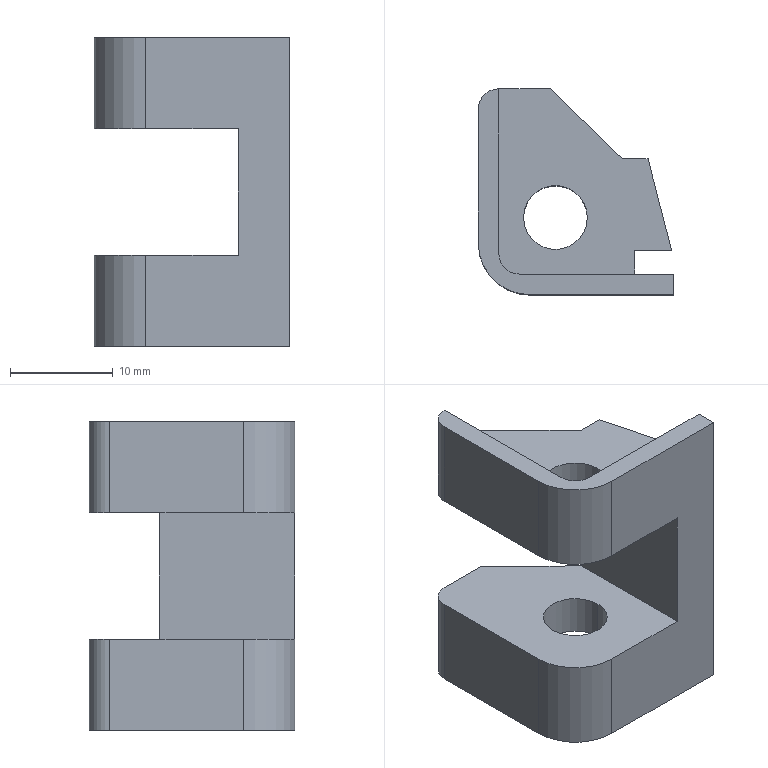Part | SolidWorks | features BaseBody 1 | 1 solid | 32 faces | box 19 x 20 x 30 mm | volume 3284 mm3 | plane 22 | cylinder 10 | commonest cylinder face diameters 4 x4 6.2 x4 10 x2
STEP:
#1=CARTESIAN_POINT('',(10.6,-12.5,-8.85));
#2=VERTEX_POINT('',#1);
#3=CARTESIAN_POINT('',(4.4,-12.5,-8.85));
#4=VERTEX_POINT('',#3);
#5=CARTESIAN_POINT('',(7.5,-12.5,-8.85));
#6=DIRECTION('',(0.,0.,-1.));
#7=DIRECTION('',(1.,0.,0.));
#8=AXIS2_PLACEMENT_3D('',#5,#6,#7);
#9=CIRCLE('',#8,3.1);
#10=EDGE_CURVE('',#2,#4,#9,.T.);
#11=ORIENTED_EDGE('',*,*,#10,.T.);
#12=CARTESIAN_POINT('',(4.4,-12.5,-5.));
#13=VERTEX_POINT('',#12);
#14=CARTESIAN_POINT('',(4.4,-12.5,-30.));
#15=DIRECTION('',(0.,0.,1.));
#16=VECTOR('',#15,1000.);
#17=LINE('',#14,#16);
#18=EDGE_CURVE('',#4,#13,#17,.T.);
#19=ORIENTED_EDGE('',*,*,#18,.T.);
#20=CARTESIAN_POINT('',(10.6,-12.5,-5.));
#21=VERTEX_POINT('',#20);
#22=CARTESIAN_POINT('',(7.5,-12.5,-5.));
#23=DIRECTION('',(0.,0.,-1.));
#24=DIRECTION('',(1.,0.,0.));
#25=AXIS2_PLACEMENT_3D('',#22,#23,#24);
#26=CIRCLE('',#25,3.1);
#27=EDGE_CURVE('',#21,#13,#26,.T.);
#28=ORIENTED_EDGE('',*,*,#27,.F.);
#29=CARTESIAN_POINT('',(10.6,-12.5,-30.));
#30=DIRECTION('',(0.,0.,1.));
#31=VECTOR('',#30,1000.);
#32=LINE('',#29,#31);
#33=EDGE_CURVE('',#2,#21,#32,.T.);
#34=ORIENTED_EDGE('',*,*,#33,.F.);
#35=EDGE_LOOP('',(#11,#19,#28,#34));
#36=FACE_OUTER_BOUND('',#35,.T.);
#37=CARTESIAN_POINT('',(7.5,-12.5,-30.));
#38=DIRECTION('',(0.,0.,1.));
#39=DIRECTION('',(1.,0.,0.));
#40=AXIS2_PLACEMENT_3D('',#37,#38,#39);
#41=CYLINDRICAL_SURFACE('',#40,3.1);
#42=ADVANCED_FACE('',(#36),#41,.F.);
#43=CARTESIAN_POINT('',(4.4,-12.5,-25.));
#44=VERTEX_POINT('',#43);
#45=CARTESIAN_POINT('',(10.6,-12.5,-25.));
#46=VERTEX_POINT('',#45);
#47=CARTESIAN_POINT('',(7.5,-12.5,-25.));
#48=DIRECTION('',(0.,0.,1.));
#49=DIRECTION('',(1.,0.,0.));
#50=AXIS2_PLACEMENT_3D('',#47,#48,#49);
#51=CIRCLE('',#50,3.1);
#52=EDGE_CURVE('',#44,#46,#51,.T.);
#53=ORIENTED_EDGE('',*,*,#52,.F.);
#54=CARTESIAN_POINT('',(4.4,-12.5,-21.15));
#55=VERTEX_POINT('',#54);
#56=CARTESIAN_POINT('',(4.4,-12.5,-30.));
#57=DIRECTION('',(0.,0.,1.));
#58=VECTOR('',#57,1000.);
#59=LINE('',#56,#58);
#60=EDGE_CURVE('',#44,#55,#59,.T.);
#61=ORIENTED_EDGE('',*,*,#60,.T.);
#62=CARTESIAN_POINT('',(10.6,-12.5,-21.15));
#63=VERTEX_POINT('',#62);
#64=CARTESIAN_POINT('',(7.5,-12.5,-21.15));
#65=DIRECTION('',(0.,0.,-1.));
#66=DIRECTION('',(1.,0.,0.));
#67=AXIS2_PLACEMENT_3D('',#64,#65,#66);
#68=CIRCLE('',#67,3.1);
#69=EDGE_CURVE('',#63,#55,#68,.T.);
#70=ORIENTED_EDGE('',*,*,#69,.F.);
#71=CARTESIAN_POINT('',(10.6,-12.5,-30.));
#72=DIRECTION('',(0.,0.,1.));
#73=VECTOR('',#72,1000.);
#74=LINE('',#71,#73);
#75=EDGE_CURVE('',#46,#63,#74,.T.);
#76=ORIENTED_EDGE('',*,*,#75,.F.);
#77=EDGE_LOOP('',(#53,#61,#70,#76));
#78=FACE_OUTER_BOUND('',#77,.T.);
#79=CARTESIAN_POINT('',(7.5,-12.5,-30.));
#80=DIRECTION('',(0.,0.,1.));
#81=DIRECTION('',(1.,0.,0.));
#82=AXIS2_PLACEMENT_3D('',#79,#80,#81);
#83=CYLINDRICAL_SURFACE('',#82,3.1);
#84=ADVANCED_FACE('',(#78),#83,.F.);
#85=CARTESIAN_POINT('',(5.,-20.,-8.85));
#86=VERTEX_POINT('',#85);
#87=CARTESIAN_POINT('',(14.,-20.,-8.85));
#88=VERTEX_POINT('',#87);
#89=CARTESIAN_POINT('',(0.,-20.,-8.85));
#90=DIRECTION('',(1.,0.,0.));
#91=VECTOR('',#90,1000.);
#92=LINE('',#89,#91);
#93=EDGE_CURVE('',#86,#88,#92,.T.);
#94=ORIENTED_EDGE('',*,*,#93,.T.);
#95=CARTESIAN_POINT('',(14.,-20.,-21.15));
#96=VERTEX_POINT('',#95);
#97=CARTESIAN_POINT('',(14.,-20.,-30.));
#98=DIRECTION('',(0.,0.,-1.));
#99=VECTOR('',#98,1000.);
#100=LINE('',#97,#99);
#101=EDGE_CURVE('',#88,#96,#100,.T.);
#102=ORIENTED_EDGE('',*,*,#101,.T.);
#103=CARTESIAN_POINT('',(5.,-20.,-21.15));
#104=VERTEX_POINT('',#103);
#105=CARTESIAN_POINT('',(0.,-20.,-21.15));
#106=DIRECTION('',(-1.,0.,0.));
#107=VECTOR('',#106,1000.);
#108=LINE('',#105,#107);
#109=EDGE_CURVE('',#96,#104,#108,.T.);
#110=ORIENTED_EDGE('',*,*,#109,.T.);
#111=CARTESIAN_POINT('',(5.,-20.,-30.));
#112=VERTEX_POINT('',#111);
#113=CARTESIAN_POINT('',(5.,-20.,-30.));
#114=DIRECTION('',(0.,0.,-1.));
#115=VECTOR('',#114,1000.);
#116=LINE('',#113,#115);
#117=EDGE_CURVE('',#104,#112,#116,.T.);
#118=ORIENTED_EDGE('',*,*,#117,.T.);
#119=CARTESIAN_POINT('',(19.,-20.,-30.));
#120=VERTEX_POINT('',#119);
#121=CARTESIAN_POINT('',(0.,-20.,-30.));
#122=DIRECTION('',(1.,0.,0.));
#123=VECTOR('',#122,1000.);
#124=LINE('',#121,#123);
#125=EDGE_CURVE('',#112,#120,#124,.T.);
#126=ORIENTED_EDGE('',*,*,#125,.T.);
#127=CARTESIAN_POINT('',(19.,-20.,0.));
#128=VERTEX_POINT('',#127);
#129=CARTESIAN_POINT('',(19.,-20.,-30.));
#130=DIRECTION('',(0.,0.,1.));
#131=VECTOR('',#130,1000.);
#132=LINE('',#129,#131);
#133=EDGE_CURVE('',#120,#128,#132,.T.);
#134=ORIENTED_EDGE('',*,*,#133,.T.);
#135=CARTESIAN_POINT('',(5.,-20.,0.));
#136=VERTEX_POINT('',#135);
#137=CARTESIAN_POINT('',(0.,-20.,0.));
#138=DIRECTION('',(-1.,0.,0.));
#139=VECTOR('',#138,1000.);
#140=LINE('',#137,#139);
#141=EDGE_CURVE('',#128,#136,#140,.T.);
#142=ORIENTED_EDGE('',*,*,#141,.T.);
#143=CARTESIAN_POINT('',(5.,-20.,-30.));
#144=DIRECTION('',(0.,0.,-1.));
#145=VECTOR('',#144,1000.);
#146=LINE('',#143,#145);
#147=EDGE_CURVE('',#136,#86,#146,.T.);
#148=ORIENTED_EDGE('',*,*,#147,.T.);
#149=EDGE_LOOP('',(#94,#102,#110,#118,#126,#134,#142,#148));
#150=FACE_OUTER_BOUND('',#149,.T.);
#151=CARTESIAN_POINT('',(0.,-20.,-30.));
#152=DIRECTION('',(0.,-1.,0.));
#153=DIRECTION('',(0.,0.,-1.));
#154=AXIS2_PLACEMENT_3D('',#151,#152,#153);
#155=PLANE('',#154);
#156=ADVANCED_FACE('',(#150),#155,.T.);
#157=CARTESIAN_POINT('',(14.,-6.8,-8.85));
#158=VERTEX_POINT('',#157);
#159=CARTESIAN_POINT('',(14.,0.,-8.85));
#160=DIRECTION('',(0.,1.,0.));
#161=VECTOR('',#160,1000.);
#162=LINE('',#159,#161);
#163=EDGE_CURVE('',#88,#158,#162,.T.);
#164=ORIENTED_EDGE('',*,*,#163,.T.);
#165=CARTESIAN_POINT('',(14.,-6.8,-21.15));
#166=VERTEX_POINT('',#165);
#167=CARTESIAN_POINT('',(14.,-6.8,-8.85));
#168=DIRECTION('',(0.,0.,-1.));
#169=VECTOR('',#168,1000.);
#170=LINE('',#167,#169);
#171=EDGE_CURVE('',#158,#166,#170,.T.);
#172=ORIENTED_EDGE('',*,*,#171,.T.);
#173=CARTESIAN_POINT('',(14.,0.,-21.15));
#174=DIRECTION('',(0.,-1.,0.));
#175=VECTOR('',#174,1000.);
#176=LINE('',#173,#175);
#177=EDGE_CURVE('',#166,#96,#176,.T.);
#178=ORIENTED_EDGE('',*,*,#177,.T.);
#179=ORIENTED_EDGE('',*,*,#101,.F.);
#180=EDGE_LOOP('',(#164,#172,#178,#179));
#181=FACE_OUTER_BOUND('',#180,.T.);
#182=CARTESIAN_POINT('',(14.,0.,-8.85));
#183=DIRECTION('',(-1.,0.,0.));
#184=DIRECTION('',(0.,-1.,0.));
#185=AXIS2_PLACEMENT_3D('',#182,#183,#184);
#186=PLANE('',#185);
#187=ADVANCED_FACE('',(#181),#186,.T.);
#188=CARTESIAN_POINT('',(2.,0.,-8.85));
#189=VERTEX_POINT('',#188);
#190=CARTESIAN_POINT('',(0.,-2.,-8.85));
#191=VERTEX_POINT('',#190);
#192=CARTESIAN_POINT('',(2.,-2.,-8.85));
#193=DIRECTION('',(0.,0.,1.));
#194=DIRECTION('',(1.,0.,0.));
#195=AXIS2_PLACEMENT_3D('',#192,#193,#194);
#196=CIRCLE('',#195,2.);
#197=EDGE_CURVE('',#189,#191,#196,.T.);
#198=ORIENTED_EDGE('',*,*,#197,.F.);
#199=CARTESIAN_POINT('',(7.,0.,-8.85));
#200=VERTEX_POINT('',#199);
#201=CARTESIAN_POINT('',(0.,0.,-8.85));
#202=DIRECTION('',(-1.,0.,0.));
#203=VECTOR('',#202,1000.);
#204=LINE('',#201,#203);
#205=EDGE_CURVE('',#200,#189,#204,.T.);
#206=ORIENTED_EDGE('',*,*,#205,.F.);
#207=CARTESIAN_POINT('',(14.,-6.8,-8.85));
#208=DIRECTION('',(-0.7173,0.6968,0.));
#209=VECTOR('',#208,1000.);
#210=LINE('',#207,#209);
#211=EDGE_CURVE('',#158,#200,#210,.T.);
#212=ORIENTED_EDGE('',*,*,#211,.F.);
#213=ORIENTED_EDGE('',*,*,#163,.F.);
#214=ORIENTED_EDGE('',*,*,#93,.F.);
#215=CARTESIAN_POINT('',(0.,-15.,-8.85));
#216=VERTEX_POINT('',#215);
#217=CARTESIAN_POINT('',(5.,-15.,-8.85));
#218=DIRECTION('',(0.,0.,1.));
#219=DIRECTION('',(1.,0.,0.));
#220=AXIS2_PLACEMENT_3D('',#217,#218,#219);
#221=CIRCLE('',#220,5.);
#222=EDGE_CURVE('',#216,#86,#221,.T.);
#223=ORIENTED_EDGE('',*,*,#222,.F.);
#224=CARTESIAN_POINT('',(0.,0.,-8.85));
#225=DIRECTION('',(0.,-1.,0.));
#226=VECTOR('',#225,1000.);
#227=LINE('',#224,#226);
#228=EDGE_CURVE('',#191,#216,#227,.T.);
#229=ORIENTED_EDGE('',*,*,#228,.F.);
#230=EDGE_LOOP('',(#198,#206,#212,#213,#214,#223,#229));
#231=FACE_OUTER_BOUND('',#230,.T.);
#232=ORIENTED_EDGE('',*,*,#10,.F.);
#233=CARTESIAN_POINT('',(7.5,-12.5,-8.85));
#234=DIRECTION('',(0.,0.,-1.));
#235=DIRECTION('',(1.,0.,0.));
#236=AXIS2_PLACEMENT_3D('',#233,#234,#235);
#237=CIRCLE('',#236,3.1);
#238=EDGE_CURVE('',#4,#2,#237,.T.);
#239=ORIENTED_EDGE('',*,*,#238,.F.);
#240=EDGE_LOOP('',(#232,#239));
#241=FACE_BOUND('',#240,.T.);
#242=CARTESIAN_POINT('',(0.,0.,-8.85));
#243=DIRECTION('',(0.,0.,1.));
#244=DIRECTION('',(1.,0.,0.));
#245=AXIS2_PLACEMENT_3D('',#242,#243,#244);
#246=PLANE('',#245);
#247=ADVANCED_FACE('',(#231,#241),#246,.F.);
#248=CARTESIAN_POINT('',(0.,-15.,0.));
#249=VERTEX_POINT('',#248);
#250=CARTESIAN_POINT('',(5.,-15.,0.));
#251=DIRECTION('',(0.,0.,-1.));
#252=DIRECTION('',(1.,0.,0.));
#253=AXIS2_PLACEMENT_3D('',#250,#251,#252);
#254=CIRCLE('',#253,5.);
#255=EDGE_CURVE('',#136,#249,#254,.T.);
#256=ORIENTED_EDGE('',*,*,#255,.T.);
#257=CARTESIAN_POINT('',(0.,-15.,-30.));
#258=DIRECTION('',(0.,0.,-1.));
#259=VECTOR('',#258,1000.);
#260=LINE('',#257,#259);
#261=EDGE_CURVE('',#249,#216,#260,.T.);
#262=ORIENTED_EDGE('',*,*,#261,.T.);
#263=ORIENTED_EDGE('',*,*,#222,.T.);
#264=ORIENTED_EDGE('',*,*,#147,.F.);
#265=EDGE_LOOP('',(#256,#262,#263,#264));
#266=FACE_OUTER_BOUND('',#265,.T.);
#267=CARTESIAN_POINT('',(5.,-15.,-30.));
#268=DIRECTION('',(0.,0.,1.));
#269=DIRECTION('',(1.,0.,0.));
#270=AXIS2_PLACEMENT_3D('',#267,#268,#269);
#271=CYLINDRICAL_SURFACE('',#270,5.);
#272=ADVANCED_FACE('',(#266),#271,.T.);
#273=CARTESIAN_POINT('',(0.,-2.,0.));
#274=VERTEX_POINT('',#273);
#275=CARTESIAN_POINT('',(2.,0.,0.));
#276=VERTEX_POINT('',#275);
#277=CARTESIAN_POINT('',(2.,-2.,0.));
#278=DIRECTION('',(0.,0.,-1.));
#279=DIRECTION('',(1.,0.,0.));
#280=AXIS2_PLACEMENT_3D('',#277,#278,#279);
#281=CIRCLE('',#280,2.);
#282=EDGE_CURVE('',#274,#276,#281,.T.);
#283=ORIENTED_EDGE('',*,*,#282,.F.);
#284=CARTESIAN_POINT('',(0.,0.,0.));
#285=DIRECTION('',(0.,1.,0.));
#286=VECTOR('',#285,1000.);
#287=LINE('',#284,#286);
#288=EDGE_CURVE('',#249,#274,#287,.T.);
#289=ORIENTED_EDGE('',*,*,#288,.F.);
#290=ORIENTED_EDGE('',*,*,#255,.F.);
#291=ORIENTED_EDGE('',*,*,#141,.F.);
#292=CARTESIAN_POINT('',(19.,-18.,0.));
#293=VERTEX_POINT('',#292);
#294=CARTESIAN_POINT('',(19.,0.,0.));
#295=DIRECTION('',(0.,-1.,0.));
#296=VECTOR('',#295,1000.);
#297=LINE('',#294,#296);
#298=EDGE_CURVE('',#293,#128,#297,.T.);
#299=ORIENTED_EDGE('',*,*,#298,.F.);
#300=CARTESIAN_POINT('',(4.,-18.,0.));
#301=VERTEX_POINT('',#300);
#302=CARTESIAN_POINT('',(0.,-18.,0.));
#303=DIRECTION('',(1.,0.,0.));
#304=VECTOR('',#303,1000.);
#305=LINE('',#302,#304);
#306=EDGE_CURVE('',#301,#293,#305,.T.);
#307=ORIENTED_EDGE('',*,*,#306,.F.);
#308=CARTESIAN_POINT('',(2.,-16.,0.));
#309=VERTEX_POINT('',#308);
#310=CARTESIAN_POINT('',(4.,-16.,0.));
#311=DIRECTION('',(0.,0.,1.));
#312=DIRECTION('',(-1.,0.,0.));
#313=AXIS2_PLACEMENT_3D('',#310,#311,#312);
#314=CIRCLE('',#313,2.);
#315=EDGE_CURVE('',#309,#301,#314,.T.);
#316=ORIENTED_EDGE('',*,*,#315,.F.);
#317=CARTESIAN_POINT('',(2.,0.,0.));
#318=DIRECTION('',(0.,-1.,0.));
#319=VECTOR('',#318,1000.);
#320=LINE('',#317,#319);
#321=EDGE_CURVE('',#276,#309,#320,.T.);
#322=ORIENTED_EDGE('',*,*,#321,.F.);
#323=EDGE_LOOP('',(#283,#289,#290,#291,#299,#307,#316,#322));
#324=FACE_OUTER_BOUND('',#323,.T.);
#325=CARTESIAN_POINT('',(0.,0.,0.));
#326=DIRECTION('',(0.,0.,-1.));
#327=DIRECTION('',(-1.,0.,0.));
#328=AXIS2_PLACEMENT_3D('',#325,#326,#327);
#329=PLANE('',#328);
#330=ADVANCED_FACE('',(#324),#329,.F.);
#331=CARTESIAN_POINT('',(19.,-18.,-30.));
#332=VERTEX_POINT('',#331);
#333=CARTESIAN_POINT('',(19.,-18.,-30.));
#334=DIRECTION('',(0.,1.,0.));
#335=VECTOR('',#334,1000.);
#336=LINE('',#333,#335);
#337=EDGE_CURVE('',#120,#332,#336,.T.);
#338=ORIENTED_EDGE('',*,*,#337,.T.);
#339=CARTESIAN_POINT('',(19.,-18.,-30.));
#340=DIRECTION('',(0.,0.,1.));
#341=VECTOR('',#340,1000.);
#342=LINE('',#339,#341);
#343=EDGE_CURVE('',#332,#293,#342,.T.);
#344=ORIENTED_EDGE('',*,*,#343,.T.);
#345=ORIENTED_EDGE('',*,*,#298,.T.);
#346=ORIENTED_EDGE('',*,*,#133,.F.);
#347=EDGE_LOOP('',(#338,#344,#345,#346));
#348=FACE_OUTER_BOUND('',#347,.T.);
#349=CARTESIAN_POINT('',(19.,-18.,-30.));
#350=DIRECTION('',(1.,0.,0.));
#351=DIRECTION('',(0.,0.,-1.));
#352=AXIS2_PLACEMENT_3D('',#349,#350,#351);
#353=PLANE('',#352);
#354=ADVANCED_FACE('',(#348),#353,.T.);
#355=ORIENTED_EDGE('',*,*,#125,.F.);
#356=CARTESIAN_POINT('',(0.,-15.,-30.));
#357=VERTEX_POINT('',#356);
#358=CARTESIAN_POINT('',(5.,-15.,-30.));
#359=DIRECTION('',(0.,0.,-1.));
#360=DIRECTION('',(1.,0.,0.));
#361=AXIS2_PLACEMENT_3D('',#358,#359,#360);
#362=CIRCLE('',#361,5.);
#363=EDGE_CURVE('',#112,#357,#362,.T.);
#364=ORIENTED_EDGE('',*,*,#363,.T.);
#365=CARTESIAN_POINT('',(0.,-2.,-30.));
#366=VERTEX_POINT('',#365);
#367=CARTESIAN_POINT('',(0.,0.,-30.));
#368=DIRECTION('',(0.,1.,0.));
#369=VECTOR('',#368,1000.);
#370=LINE('',#367,#369);
#371=EDGE_CURVE('',#357,#366,#370,.T.);
#372=ORIENTED_EDGE('',*,*,#371,.T.);
#373=CARTESIAN_POINT('',(2.,0.,-30.));
#374=VERTEX_POINT('',#373);
#375=CARTESIAN_POINT('',(2.,-2.,-30.));
#376=DIRECTION('',(0.,0.,-1.));
#377=DIRECTION('',(1.,0.,0.));
#378=AXIS2_PLACEMENT_3D('',#375,#376,#377);
#379=CIRCLE('',#378,2.);
#380=EDGE_CURVE('',#366,#374,#379,.T.);
#381=ORIENTED_EDGE('',*,*,#380,.T.);
#382=CARTESIAN_POINT('',(2.,-16.,-30.));
#383=VERTEX_POINT('',#382);
#384=CARTESIAN_POINT('',(2.,0.,-30.));
#385=DIRECTION('',(0.,-1.,0.));
#386=VECTOR('',#385,1000.);
#387=LINE('',#384,#386);
#388=EDGE_CURVE('',#374,#383,#387,.T.);
#389=ORIENTED_EDGE('',*,*,#388,.T.);
#390=CARTESIAN_POINT('',(4.,-18.,-30.));
#391=VERTEX_POINT('',#390);
#392=CARTESIAN_POINT('',(4.,-16.,-30.));
#393=DIRECTION('',(0.,0.,1.));
#394=DIRECTION('',(-1.,0.,0.));
#395=AXIS2_PLACEMENT_3D('',#392,#393,#394);
#396=CIRCLE('',#395,2.);
#397=EDGE_CURVE('',#383,#391,#396,.T.);
#398=ORIENTED_EDGE('',*,*,#397,.T.);
#399=CARTESIAN_POINT('',(0.,-18.,-30.));
#400=DIRECTION('',(1.,0.,0.));
#401=VECTOR('',#400,1000.);
#402=LINE('',#399,#401);
#403=EDGE_CURVE('',#391,#332,#402,.T.);
#404=ORIENTED_EDGE('',*,*,#403,.T.);
#405=ORIENTED_EDGE('',*,*,#337,.F.);
#406=EDGE_LOOP('',(#355,#364,#372,#381,#389,#398,#404,#405));
#407=FACE_OUTER_BOUND('',#406,.T.);
#408=CARTESIAN_POINT('',(0.,0.,-30.));
#409=DIRECTION('',(0.,0.,-1.));
#410=DIRECTION('',(-1.,0.,0.));
#411=AXIS2_PLACEMENT_3D('',#408,#409,#410);
#412=PLANE('',#411);
#413=ADVANCED_FACE('',(#407),#412,.T.);
#414=CARTESIAN_POINT('',(0.,-15.,-21.15));
#415=VERTEX_POINT('',#414);
#416=CARTESIAN_POINT('',(5.,-15.,-21.15));
#417=DIRECTION('',(0.,0.,-1.));
#418=DIRECTION('',(1.,0.,0.));
#419=AXIS2_PLACEMENT_3D('',#416,#417,#418);
#420=CIRCLE('',#419,5.);
#421=EDGE_CURVE('',#104,#415,#420,.T.);
#422=ORIENTED_EDGE('',*,*,#421,.T.);
#423=CARTESIAN_POINT('',(0.,-15.,-30.));
#424=DIRECTION('',(0.,0.,-1.));
#425=VECTOR('',#424,1000.);
#426=LINE('',#423,#425);
#427=EDGE_CURVE('',#415,#357,#426,.T.);
#428=ORIENTED_EDGE('',*,*,#427,.T.);
#429=ORIENTED_EDGE('',*,*,#363,.F.);
#430=ORIENTED_EDGE('',*,*,#117,.F.);
#431=EDGE_LOOP('',(#422,#428,#429,#430));
#432=FACE_OUTER_BOUND('',#431,.T.);
#433=CARTESIAN_POINT('',(5.,-15.,-30.));
#434=DIRECTION('',(0.,0.,1.));
#435=DIRECTION('',(1.,0.,0.));
#436=AXIS2_PLACEMENT_3D('',#433,#434,#435);
#437=CYLINDRICAL_SURFACE('',#436,5.);
#438=ADVANCED_FACE('',(#432),#437,.T.);
#439=ORIENTED_EDGE('',*,*,#177,.F.);
#440=CARTESIAN_POINT('',(7.,0.,-21.15));
#441=VERTEX_POINT('',#440);
#442=CARTESIAN_POINT('',(14.,-6.8,-21.15));
#443=DIRECTION('',(-0.7173,0.6968,0.));
#444=VECTOR('',#443,1000.);
#445=LINE('',#442,#444);
#446=EDGE_CURVE('',#166,#441,#445,.T.);
#447=ORIENTED_EDGE('',*,*,#446,.T.);
#448=CARTESIAN_POINT('',(2.,0.,-21.15));
#449=VERTEX_POINT('',#448);
#450=CARTESIAN_POINT('',(0.,0.,-21.15));
#451=DIRECTION('',(-1.,0.,0.));
#452=VECTOR('',#451,1000.);
#453=LINE('',#450,#452);
#454=EDGE_CURVE('',#441,#449,#453,.T.);
#455=ORIENTED_EDGE('',*,*,#454,.T.);
#456=CARTESIAN_POINT('',(0.,-2.,-21.15));
#457=VERTEX_POINT('',#456);
#458=CARTESIAN_POINT('',(2.,-2.,-21.15));
#459=DIRECTION('',(0.,0.,1.));
#460=DIRECTION('',(1.,0.,0.));
#461=AXIS2_PLACEMENT_3D('',#458,#459,#460);
#462=CIRCLE('',#461,2.);
#463=EDGE_CURVE('',#449,#457,#462,.T.);
#464=ORIENTED_EDGE('',*,*,#463,.T.);
#465=CARTESIAN_POINT('',(0.,0.,-21.15));
#466=DIRECTION('',(0.,-1.,0.));
#467=VECTOR('',#466,1000.);
#468=LINE('',#465,#467);
#469=EDGE_CURVE('',#457,#415,#468,.T.);
#470=ORIENTED_EDGE('',*,*,#469,.T.);
#471=ORIENTED_EDGE('',*,*,#421,.F.);
#472=ORIENTED_EDGE('',*,*,#109,.F.);
#473=EDGE_LOOP('',(#439,#447,#455,#464,#470,#471,#472));
#474=FACE_OUTER_BOUND('',#473,.T.);
#475=ORIENTED_EDGE('',*,*,#69,.T.);
#476=CARTESIAN_POINT('',(7.5,-12.5,-21.15));
#477=DIRECTION('',(0.,0.,-1.));
#478=DIRECTION('',(1.,0.,0.));
#479=AXIS2_PLACEMENT_3D('',#476,#477,#478);
#480=CIRCLE('',#479,3.1);
#481=EDGE_CURVE('',#55,#63,#480,.T.);
#482=ORIENTED_EDGE('',*,*,#481,.T.);
#483=EDGE_LOOP('',(#475,#482));
#484=FACE_BOUND('',#483,.T.);
#485=CARTESIAN_POINT('',(0.,0.,-21.15));
#486=DIRECTION('',(0.,0.,1.));
#487=DIRECTION('',(1.,0.,0.));
#488=AXIS2_PLACEMENT_3D('',#485,#486,#487);
#489=PLANE('',#488);
#490=ADVANCED_FACE('',(#474,#484),#489,.T.);
#491=CARTESIAN_POINT('',(16.5,-6.8,-5.));
#492=VERTEX_POINT('',#491);
#493=CARTESIAN_POINT('',(16.5,-6.8,-25.));
#494=VERTEX_POINT('',#493);
#495=CARTESIAN_POINT('',(16.5,-6.8,-25.));
#496=DIRECTION('',(0.,0.,-1.));
#497=VECTOR('',#496,1000.);
#498=LINE('',#495,#497);
#499=EDGE_CURVE('',#492,#494,#498,.T.);
#500=ORIENTED_EDGE('',*,*,#499,.T.);
#501=CARTESIAN_POINT('',(14.,-6.8,-25.));
#502=VERTEX_POINT('',#501);
#503=CARTESIAN_POINT('',(14.,-6.8,-25.));
#504=DIRECTION('',(-1.,0.,0.));
#505=VECTOR('',#504,1000.);
#506=LINE('',#503,#505);
#507=EDGE_CURVE('',#494,#502,#506,.T.);
#508=ORIENTED_EDGE('',*,*,#507,.T.);
#509=CARTESIAN_POINT('',(14.,-6.8,-25.));
#510=DIRECTION('',(0.,0.,1.));
#511=VECTOR('',#510,1000.);
#512=LINE('',#509,#511);
#513=EDGE_CURVE('',#502,#166,#512,.T.);
#514=ORIENTED_EDGE('',*,*,#513,.T.);
#515=ORIENTED_EDGE('',*,*,#171,.F.);
#516=CARTESIAN_POINT('',(14.,-6.8,-5.));
#517=VERTEX_POINT('',#516);
#518=CARTESIAN_POINT('',(14.,-6.8,-25.));
#519=DIRECTION('',(0.,0.,1.));
#520=VECTOR('',#519,1000.);
#521=LINE('',#518,#520);
#522=EDGE_CURVE('',#158,#517,#521,.T.);
#523=ORIENTED_EDGE('',*,*,#522,.T.);
#524=CARTESIAN_POINT('',(14.,-6.8,-5.));
#525=DIRECTION('',(1.,0.,0.));
#526=VECTOR('',#525,1000.);
#527=LINE('',#524,#526);
#528=EDGE_CURVE('',#517,#492,#527,.T.);
#529=ORIENTED_EDGE('',*,*,#528,.T.);
#530=EDGE_LOOP('',(#500,#508,#514,#515,#523,#529));
#531=FACE_OUTER_BOUND('',#530,.T.);
#532=CARTESIAN_POINT('',(14.,-6.8,-25.));
#533=DIRECTION('',(0.,1.,0.));
#534=DIRECTION('',(0.,0.,1.));
#535=AXIS2_PLACEMENT_3D('',#532,#533,#534);
#536=PLANE('',#535);
#537=ADVANCED_FACE('',(#531),#536,.T.);
#538=ORIENTED_EDGE('',*,*,#228,.T.);
#539=ORIENTED_EDGE('',*,*,#261,.F.);
#540=ORIENTED_EDGE('',*,*,#288,.T.);
#541=CARTESIAN_POINT('',(0.,-2.,-30.));
#542=DIRECTION('',(0.,0.,-1.));
#543=VECTOR('',#542,1000.);
#544=LINE('',#541,#543);
#545=EDGE_CURVE('',#274,#191,#544,.T.);
#546=ORIENTED_EDGE('',*,*,#545,.T.);
#547=EDGE_LOOP('',(#538,#539,#540,#546));
#548=FACE_OUTER_BOUND('',#547,.T.);
#549=CARTESIAN_POINT('',(0.,0.,-30.));
#550=DIRECTION('',(-1.,0.,0.));
#551=DIRECTION('',(0.,-1.,0.));
#552=AXIS2_PLACEMENT_3D('',#549,#550,#551);
#553=PLANE('',#552);
#554=ADVANCED_FACE('',(#548),#553,.T.);
#555=CARTESIAN_POINT('',(2.,0.,-5.));
#556=VERTEX_POINT('',#555);
#557=CARTESIAN_POINT('',(2.,0.,-30.));
#558=DIRECTION('',(0.,0.,-1.));
#559=VECTOR('',#558,1000.);
#560=LINE('',#557,#559);
#561=EDGE_CURVE('',#276,#556,#560,.T.);
#562=ORIENTED_EDGE('',*,*,#561,.T.);
#563=CARTESIAN_POINT('',(2.,0.,-30.));
#564=DIRECTION('',(0.,0.,-1.));
#565=VECTOR('',#564,1000.);
#566=LINE('',#563,#565);
#567=EDGE_CURVE('',#556,#189,#566,.T.);
#568=ORIENTED_EDGE('',*,*,#567,.T.);
#569=ORIENTED_EDGE('',*,*,#197,.T.);
#570=ORIENTED_EDGE('',*,*,#545,.F.);
#571=ORIENTED_EDGE('',*,*,#282,.T.);
#572=EDGE_LOOP('',(#562,#568,#569,#570,#571));
#573=FACE_OUTER_BOUND('',#572,.T.);
#574=CARTESIAN_POINT('',(2.,-2.,-30.));
#575=DIRECTION('',(0.,0.,1.));
#576=DIRECTION('',(1.,0.,0.));
#577=AXIS2_PLACEMENT_3D('',#574,#575,#576);
#578=CYLINDRICAL_SURFACE('',#577,2.);
#579=ADVANCED_FACE('',(#573),#578,.T.);
#580=CARTESIAN_POINT('',(7.,0.,-5.));
#581=VERTEX_POINT('',#580);
#582=CARTESIAN_POINT('',(0.,0.,-5.));
#583=DIRECTION('',(1.,0.,0.));
#584=VECTOR('',#583,1000.);
#585=LINE('',#582,#584);
#586=EDGE_CURVE('',#556,#581,#585,.T.);
#587=ORIENTED_EDGE('',*,*,#586,.T.);
#588=CARTESIAN_POINT('',(7.,0.,-30.));
#589=DIRECTION('',(0.,0.,-1.));
#590=VECTOR('',#589,1000.);
#591=LINE('',#588,#590);
#592=EDGE_CURVE('',#581,#200,#591,.T.);
#593=ORIENTED_EDGE('',*,*,#592,.T.);
#594=ORIENTED_EDGE('',*,*,#205,.T.);
#595=ORIENTED_EDGE('',*,*,#567,.F.);
#596=EDGE_LOOP('',(#587,#593,#594,#595));
#597=FACE_OUTER_BOUND('',#596,.T.);
#598=CARTESIAN_POINT('',(0.,0.,-30.));
#599=DIRECTION('',(0.,1.,0.));
#600=DIRECTION('',(0.,0.,1.));
#601=AXIS2_PLACEMENT_3D('',#598,#599,#600);
#602=PLANE('',#601);
#603=ADVANCED_FACE('',(#597),#602,.T.);
#604=CARTESIAN_POINT('',(7.,0.,-5.));
#605=DIRECTION('',(0.7173,-0.6968,0.));
#606=VECTOR('',#605,1000.);
#607=LINE('',#604,#606);
#608=EDGE_CURVE('',#581,#517,#607,.T.);
#609=ORIENTED_EDGE('',*,*,#608,.T.);
#610=ORIENTED_EDGE('',*,*,#522,.F.);
#611=ORIENTED_EDGE('',*,*,#211,.T.);
#612=ORIENTED_EDGE('',*,*,#592,.F.);
#613=EDGE_LOOP('',(#609,#610,#611,#612));
#614=FACE_OUTER_BOUND('',#613,.T.);
#615=CARTESIAN_POINT('',(7.,0.,-25.));
#616=DIRECTION('',(0.6968,0.7173,0.));
#617=DIRECTION('',(-0.7173,0.6968,0.));
#618=AXIS2_PLACEMENT_3D('',#615,#616,#617);
#619=PLANE('',#618);
#620=ADVANCED_FACE('',(#614),#619,.T.);
#621=ORIENTED_EDGE('',*,*,#18,.F.);
#622=ORIENTED_EDGE('',*,*,#238,.T.);
#623=ORIENTED_EDGE('',*,*,#33,.T.);
#624=CARTESIAN_POINT('',(7.5,-12.5,-5.));
#625=DIRECTION('',(0.,0.,-1.));
#626=DIRECTION('',(1.,0.,0.));
#627=AXIS2_PLACEMENT_3D('',#624,#625,#626);
#628=CIRCLE('',#627,3.1);
#629=EDGE_CURVE('',#13,#21,#628,.T.);
#630=ORIENTED_EDGE('',*,*,#629,.F.);
#631=EDGE_LOOP('',(#621,#622,#623,#630));
#632=FACE_OUTER_BOUND('',#631,.T.);
#633=CARTESIAN_POINT('',(7.5,-12.5,-30.));
#634=DIRECTION('',(0.,0.,1.));
#635=DIRECTION('',(1.,0.,0.));
#636=AXIS2_PLACEMENT_3D('',#633,#634,#635);
#637=CYLINDRICAL_SURFACE('',#636,3.1);
#638=ADVANCED_FACE('',(#632),#637,.F.);
#639=CARTESIAN_POINT('',(2.,-16.,-5.));
#640=VERTEX_POINT('',#639);
#641=CARTESIAN_POINT('',(2.,0.,-5.));
#642=DIRECTION('',(0.,1.,0.));
#643=VECTOR('',#642,1000.);
#644=LINE('',#641,#643);
#645=EDGE_CURVE('',#640,#556,#644,.T.);
#646=ORIENTED_EDGE('',*,*,#645,.T.);
#647=ORIENTED_EDGE('',*,*,#561,.F.);
#648=ORIENTED_EDGE('',*,*,#321,.T.);
#649=CARTESIAN_POINT('',(2.,-16.,-30.));
#650=DIRECTION('',(0.,0.,-1.));
#651=VECTOR('',#650,1000.);
#652=LINE('',#649,#651);
#653=EDGE_CURVE('',#309,#640,#652,.T.);
#654=ORIENTED_EDGE('',*,*,#653,.T.);
#655=EDGE_LOOP('',(#646,#647,#648,#654));
#656=FACE_OUTER_BOUND('',#655,.T.);
#657=CARTESIAN_POINT('',(2.,0.,-30.));
#658=DIRECTION('',(1.,0.,0.));
#659=DIRECTION('',(0.,0.,-1.));
#660=AXIS2_PLACEMENT_3D('',#657,#658,#659);
#661=PLANE('',#660);
#662=ADVANCED_FACE('',(#656),#661,.T.);
#663=ORIENTED_EDGE('',*,*,#306,.T.);
#664=ORIENTED_EDGE('',*,*,#343,.F.);
#665=ORIENTED_EDGE('',*,*,#403,.F.);
#666=CARTESIAN_POINT('',(4.,-18.,-25.));
#667=VERTEX_POINT('',#666);
#668=CARTESIAN_POINT('',(4.,-18.,-30.));
#669=DIRECTION('',(0.,0.,1.));
#670=VECTOR('',#669,1000.);
#671=LINE('',#668,#670);
#672=EDGE_CURVE('',#391,#667,#671,.T.);
#673=ORIENTED_EDGE('',*,*,#672,.T.);
#674=CARTESIAN_POINT('',(15.2,-18.,-25.));
#675=VERTEX_POINT('',#674);
#676=CARTESIAN_POINT('',(2.,-18.,-25.));
#677=DIRECTION('',(1.,0.,0.));
#678=VECTOR('',#677,1000.);
#679=LINE('',#676,#678);
#680=EDGE_CURVE('',#667,#675,#679,.T.);
#681=ORIENTED_EDGE('',*,*,#680,.T.);
#682=CARTESIAN_POINT('',(15.2,-18.,-5.));
#683=VERTEX_POINT('',#682);
#684=CARTESIAN_POINT('',(15.2,-18.,-30.));
#685=DIRECTION('',(0.,0.,1.));
#686=VECTOR('',#685,1000.);
#687=LINE('',#684,#686);
#688=EDGE_CURVE('',#675,#683,#687,.T.);
#689=ORIENTED_EDGE('',*,*,#688,.T.);
#690=CARTESIAN_POINT('',(4.,-18.,-5.));
#691=VERTEX_POINT('',#690);
#692=CARTESIAN_POINT('',(2.,-18.,-5.));
#693=DIRECTION('',(-1.,0.,0.));
#694=VECTOR('',#693,1000.);
#695=LINE('',#692,#694);
#696=EDGE_CURVE('',#683,#691,#695,.T.);
#697=ORIENTED_EDGE('',*,*,#696,.T.);
#698=CARTESIAN_POINT('',(4.,-18.,-30.));
#699=DIRECTION('',(0.,0.,1.));
#700=VECTOR('',#699,1000.);
#701=LINE('',#698,#700);
#702=EDGE_CURVE('',#691,#301,#701,.T.);
#703=ORIENTED_EDGE('',*,*,#702,.T.);
#704=EDGE_LOOP('',(#663,#664,#665,#673,#681,#689,#697,#703));
#705=FACE_OUTER_BOUND('',#704,.T.);
#706=CARTESIAN_POINT('',(2.,-18.,-30.));
#707=DIRECTION('',(0.,1.,0.));
#708=DIRECTION('',(0.,0.,1.));
#709=AXIS2_PLACEMENT_3D('',#706,#707,#708);
#710=PLANE('',#709);
#711=ADVANCED_FACE('',(#705),#710,.T.);
#712=ORIENTED_EDGE('',*,*,#653,.F.);
#713=ORIENTED_EDGE('',*,*,#315,.T.);
#714=ORIENTED_EDGE('',*,*,#702,.F.);
#715=CARTESIAN_POINT('',(4.,-16.,-5.));
#716=DIRECTION('',(0.,0.,1.));
#717=DIRECTION('',(-1.,0.,0.));
#718=AXIS2_PLACEMENT_3D('',#715,#716,#717);
#719=CIRCLE('',#718,2.);
#720=EDGE_CURVE('',#640,#691,#719,.T.);
#721=ORIENTED_EDGE('',*,*,#720,.F.);
#722=EDGE_LOOP('',(#712,#713,#714,#721));
#723=FACE_OUTER_BOUND('',#722,.T.);
#724=CARTESIAN_POINT('',(4.,-16.,-30.));
#725=DIRECTION('',(0.,0.,-1.));
#726=DIRECTION('',(-1.,0.,0.));
#727=AXIS2_PLACEMENT_3D('',#724,#725,#726);
#728=CYLINDRICAL_SURFACE('',#727,2.);
#729=ADVANCED_FACE('',(#723),#728,.F.);
#730=CARTESIAN_POINT('',(2.,-16.,-25.));
#731=VERTEX_POINT('',#730);
#732=CARTESIAN_POINT('',(2.,-16.,-30.));
#733=DIRECTION('',(0.,0.,-1.));
#734=VECTOR('',#733,1000.);
#735=LINE('',#732,#734);
#736=EDGE_CURVE('',#731,#383,#735,.T.);
#737=ORIENTED_EDGE('',*,*,#736,.F.);
#738=CARTESIAN_POINT('',(4.,-16.,-25.));
#739=DIRECTION('',(0.,0.,-1.));
#740=DIRECTION('',(-1.,0.,0.));
#741=AXIS2_PLACEMENT_3D('',#738,#739,#740);
#742=CIRCLE('',#741,2.);
#743=EDGE_CURVE('',#667,#731,#742,.T.);
#744=ORIENTED_EDGE('',*,*,#743,.F.);
#745=ORIENTED_EDGE('',*,*,#672,.F.);
#746=ORIENTED_EDGE('',*,*,#397,.F.);
#747=EDGE_LOOP('',(#737,#744,#745,#746));
#748=FACE_OUTER_BOUND('',#747,.T.);
#749=CARTESIAN_POINT('',(4.,-16.,-30.));
#750=DIRECTION('',(0.,0.,-1.));
#751=DIRECTION('',(-1.,0.,0.));
#752=AXIS2_PLACEMENT_3D('',#749,#750,#751);
#753=CYLINDRICAL_SURFACE('',#752,2.);
#754=ADVANCED_FACE('',(#748),#753,.F.);
#755=ORIENTED_EDGE('',*,*,#388,.F.);
#756=CARTESIAN_POINT('',(2.,0.,-25.));
#757=VERTEX_POINT('',#756);
#758=CARTESIAN_POINT('',(2.,0.,-30.));
#759=DIRECTION('',(0.,0.,1.));
#760=VECTOR('',#759,1000.);
#761=LINE('',#758,#760);
#762=EDGE_CURVE('',#374,#757,#761,.T.);
#763=ORIENTED_EDGE('',*,*,#762,.T.);
#764=CARTESIAN_POINT('',(2.,0.,-25.));
#765=DIRECTION('',(0.,-1.,0.));
#766=VECTOR('',#765,1000.);
#767=LINE('',#764,#766);
#768=EDGE_CURVE('',#757,#731,#767,.T.);
#769=ORIENTED_EDGE('',*,*,#768,.T.);
#770=ORIENTED_EDGE('',*,*,#736,.T.);
#771=EDGE_LOOP('',(#755,#763,#769,#770));
#772=FACE_OUTER_BOUND('',#771,.T.);
#773=CARTESIAN_POINT('',(2.,0.,-30.));
#774=DIRECTION('',(1.,0.,0.));
#775=DIRECTION('',(0.,0.,-1.));
#776=AXIS2_PLACEMENT_3D('',#773,#774,#775);
#777=PLANE('',#776);
#778=ADVANCED_FACE('',(#772),#777,.T.);
#779=CARTESIAN_POINT('',(2.,0.,-30.));
#780=DIRECTION('',(0.,0.,-1.));
#781=VECTOR('',#780,1000.);
#782=LINE('',#779,#781);
#783=EDGE_CURVE('',#449,#757,#782,.T.);
#784=ORIENTED_EDGE('',*,*,#783,.T.);
#785=ORIENTED_EDGE('',*,*,#762,.F.);
#786=ORIENTED_EDGE('',*,*,#380,.F.);
#787=CARTESIAN_POINT('',(0.,-2.,-30.));
#788=DIRECTION('',(0.,0.,1.));
#789=VECTOR('',#788,1000.);
#790=LINE('',#787,#789);
#791=EDGE_CURVE('',#366,#457,#790,.T.);
#792=ORIENTED_EDGE('',*,*,#791,.T.);
#793=ORIENTED_EDGE('',*,*,#463,.F.);
#794=EDGE_LOOP('',(#784,#785,#786,#792,#793));
#795=FACE_OUTER_BOUND('',#794,.T.);
#796=CARTESIAN_POINT('',(2.,-2.,-30.));
#797=DIRECTION('',(0.,0.,1.));
#798=DIRECTION('',(1.,0.,0.));
#799=AXIS2_PLACEMENT_3D('',#796,#797,#798);
#800=CYLINDRICAL_SURFACE('',#799,2.);
#801=ADVANCED_FACE('',(#795),#800,.T.);
#802=ORIENTED_EDGE('',*,*,#371,.F.);
#803=ORIENTED_EDGE('',*,*,#427,.F.);
#804=ORIENTED_EDGE('',*,*,#469,.F.);
#805=ORIENTED_EDGE('',*,*,#791,.F.);
#806=EDGE_LOOP('',(#802,#803,#804,#805));
#807=FACE_OUTER_BOUND('',#806,.T.);
#808=CARTESIAN_POINT('',(0.,0.,-30.));
#809=DIRECTION('',(-1.,0.,0.));
#810=DIRECTION('',(0.,-1.,0.));
#811=AXIS2_PLACEMENT_3D('',#808,#809,#810);
#812=PLANE('',#811);
#813=ADVANCED_FACE('',(#807),#812,.T.);
#814=ORIENTED_EDGE('',*,*,#513,.F.);
#815=CARTESIAN_POINT('',(7.,0.,-25.));
#816=VERTEX_POINT('',#815);
#817=CARTESIAN_POINT('',(7.,0.,-25.));
#818=DIRECTION('',(-0.7173,0.6968,0.));
#819=VECTOR('',#818,1000.);
#820=LINE('',#817,#819);
#821=EDGE_CURVE('',#502,#816,#820,.T.);
#822=ORIENTED_EDGE('',*,*,#821,.T.);
#823=CARTESIAN_POINT('',(7.,0.,-25.));
#824=DIRECTION('',(0.,0.,1.));
#825=VECTOR('',#824,1000.);
#826=LINE('',#823,#825);
#827=EDGE_CURVE('',#816,#441,#826,.T.);
#828=ORIENTED_EDGE('',*,*,#827,.T.);
#829=ORIENTED_EDGE('',*,*,#446,.F.);
#830=EDGE_LOOP('',(#814,#822,#828,#829));
#831=FACE_OUTER_BOUND('',#830,.T.);
#832=CARTESIAN_POINT('',(7.,0.,-25.));
#833=DIRECTION('',(0.6968,0.7173,0.));
#834=DIRECTION('',(-0.7173,0.6968,0.));
#835=AXIS2_PLACEMENT_3D('',#832,#833,#834);
#836=PLANE('',#835);
#837=ADVANCED_FACE('',(#831),#836,.T.);
#838=ORIENTED_EDGE('',*,*,#454,.F.);
#839=ORIENTED_EDGE('',*,*,#827,.F.);
#840=CARTESIAN_POINT('',(0.,0.,-25.));
#841=DIRECTION('',(-1.,0.,0.));
#842=VECTOR('',#841,1000.);
#843=LINE('',#840,#842);
#844=EDGE_CURVE('',#816,#757,#843,.T.);
#845=ORIENTED_EDGE('',*,*,#844,.T.);
#846=ORIENTED_EDGE('',*,*,#783,.F.);
#847=EDGE_LOOP('',(#838,#839,#845,#846));
#848=FACE_OUTER_BOUND('',#847,.T.);
#849=CARTESIAN_POINT('',(0.,0.,-30.));
#850=DIRECTION('',(0.,1.,0.));
#851=DIRECTION('',(0.,0.,1.));
#852=AXIS2_PLACEMENT_3D('',#849,#850,#851);
#853=PLANE('',#852);
#854=ADVANCED_FACE('',(#848),#853,.T.);
#855=ORIENTED_EDGE('',*,*,#60,.F.);
#856=CARTESIAN_POINT('',(7.5,-12.5,-25.));
#857=DIRECTION('',(0.,0.,1.));
#858=DIRECTION('',(1.,0.,0.));
#859=AXIS2_PLACEMENT_3D('',#856,#857,#858);
#860=CIRCLE('',#859,3.1);
#861=EDGE_CURVE('',#46,#44,#860,.T.);
#862=ORIENTED_EDGE('',*,*,#861,.F.);
#863=ORIENTED_EDGE('',*,*,#75,.T.);
#864=ORIENTED_EDGE('',*,*,#481,.F.);
#865=EDGE_LOOP('',(#855,#862,#863,#864));
#866=FACE_OUTER_BOUND('',#865,.T.);
#867=CARTESIAN_POINT('',(7.5,-12.5,-30.));
#868=DIRECTION('',(0.,0.,1.));
#869=DIRECTION('',(1.,0.,0.));
#870=AXIS2_PLACEMENT_3D('',#867,#868,#869);
#871=CYLINDRICAL_SURFACE('',#870,3.1);
#872=ADVANCED_FACE('',(#866),#871,.F.);
#873=CARTESIAN_POINT('',(18.8,-15.7,-25.));
#874=VERTEX_POINT('',#873);
#875=CARTESIAN_POINT('',(15.2,-15.7,-25.));
#876=VERTEX_POINT('',#875);
#877=CARTESIAN_POINT('',(0.,-15.7,-25.));
#878=DIRECTION('',(-1.,0.,0.));
#879=VECTOR('',#878,1000.);
#880=LINE('',#877,#879);
#881=EDGE_CURVE('',#874,#876,#880,.T.);
#882=ORIENTED_EDGE('',*,*,#881,.T.);
#883=CARTESIAN_POINT('',(15.2,0.,-25.));
#884=DIRECTION('',(0.,-1.,0.));
#885=VECTOR('',#884,1000.);
#886=LINE('',#883,#885);
#887=EDGE_CURVE('',#876,#675,#886,.T.);
#888=ORIENTED_EDGE('',*,*,#887,.T.);
#889=ORIENTED_EDGE('',*,*,#680,.F.);
#890=ORIENTED_EDGE('',*,*,#743,.T.);
#891=ORIENTED_EDGE('',*,*,#768,.F.);
#892=ORIENTED_EDGE('',*,*,#844,.F.);
#893=ORIENTED_EDGE('',*,*,#821,.F.);
#894=ORIENTED_EDGE('',*,*,#507,.F.);
#895=CARTESIAN_POINT('',(16.5,-6.8,-25.));
#896=DIRECTION('',(0.2502,-0.9682,0.));
#897=VECTOR('',#896,1000.);
#898=LINE('',#895,#897);
#899=EDGE_CURVE('',#494,#874,#898,.T.);
#900=ORIENTED_EDGE('',*,*,#899,.T.);
#901=EDGE_LOOP('',(#882,#888,#889,#890,#891,#892,#893,#894,#900));
#902=FACE_OUTER_BOUND('',#901,.T.);
#903=ORIENTED_EDGE('',*,*,#861,.T.);
#904=ORIENTED_EDGE('',*,*,#52,.T.);
#905=EDGE_LOOP('',(#903,#904));
#906=FACE_BOUND('',#905,.T.);
#907=CARTESIAN_POINT('',(0.,0.,-25.));
#908=DIRECTION('',(0.,0.,-1.));
#909=DIRECTION('',(-1.,0.,0.));
#910=AXIS2_PLACEMENT_3D('',#907,#908,#909);
#911=PLANE('',#910);
#912=ADVANCED_FACE('',(#902,#906),#911,.T.);
#913=CARTESIAN_POINT('',(18.8,-15.7,-5.));
#914=VERTEX_POINT('',#913);
#915=CARTESIAN_POINT('',(18.8,-15.7,-25.));
#916=DIRECTION('',(0.,0.,-1.));
#917=VECTOR('',#916,1000.);
#918=LINE('',#915,#917);
#919=EDGE_CURVE('',#914,#874,#918,.T.);
#920=ORIENTED_EDGE('',*,*,#919,.T.);
#921=ORIENTED_EDGE('',*,*,#899,.F.);
#922=ORIENTED_EDGE('',*,*,#499,.F.);
#923=CARTESIAN_POINT('',(16.5,-6.8,-5.));
#924=DIRECTION('',(0.2502,-0.9682,0.));
#925=VECTOR('',#924,1000.);
#926=LINE('',#923,#925);
#927=EDGE_CURVE('',#492,#914,#926,.T.);
#928=ORIENTED_EDGE('',*,*,#927,.T.);
#929=EDGE_LOOP('',(#920,#921,#922,#928));
#930=FACE_OUTER_BOUND('',#929,.T.);
#931=CARTESIAN_POINT('',(16.5,-6.8,-25.));
#932=DIRECTION('',(0.9682,0.2502,0.));
#933=DIRECTION('',(-0.2502,0.9682,0.));
#934=AXIS2_PLACEMENT_3D('',#931,#932,#933);
#935=PLANE('',#934);
#936=ADVANCED_FACE('',(#930),#935,.T.);
#937=ORIENTED_EDGE('',*,*,#720,.T.);
#938=ORIENTED_EDGE('',*,*,#696,.F.);
#939=CARTESIAN_POINT('',(15.2,-15.7,-5.));
#940=VERTEX_POINT('',#939);
#941=CARTESIAN_POINT('',(15.2,0.,-5.));
#942=DIRECTION('',(0.,-1.,0.));
#943=VECTOR('',#942,1000.);
#944=LINE('',#941,#943);
#945=EDGE_CURVE('',#940,#683,#944,.T.);
#946=ORIENTED_EDGE('',*,*,#945,.F.);
#947=CARTESIAN_POINT('',(0.,-15.7,-5.));
#948=DIRECTION('',(-1.,0.,0.));
#949=VECTOR('',#948,1000.);
#950=LINE('',#947,#949);
#951=EDGE_CURVE('',#914,#940,#950,.T.);
#952=ORIENTED_EDGE('',*,*,#951,.F.);
#953=ORIENTED_EDGE('',*,*,#927,.F.);
#954=ORIENTED_EDGE('',*,*,#528,.F.);
#955=ORIENTED_EDGE('',*,*,#608,.F.);
#956=ORIENTED_EDGE('',*,*,#586,.F.);
#957=ORIENTED_EDGE('',*,*,#645,.F.);
#958=EDGE_LOOP('',(#937,#938,#946,#952,#953,#954,#955,#956,#957));
#959=FACE_OUTER_BOUND('',#958,.T.);
#960=ORIENTED_EDGE('',*,*,#27,.T.);
#961=ORIENTED_EDGE('',*,*,#629,.T.);
#962=EDGE_LOOP('',(#960,#961));
#963=FACE_BOUND('',#962,.T.);
#964=CARTESIAN_POINT('',(0.,0.,-5.));
#965=DIRECTION('',(0.,0.,-1.));
#966=DIRECTION('',(-1.,0.,0.));
#967=AXIS2_PLACEMENT_3D('',#964,#965,#966);
#968=PLANE('',#967);
#969=ADVANCED_FACE('',(#959,#963),#968,.F.);
#970=ORIENTED_EDGE('',*,*,#688,.F.);
#971=ORIENTED_EDGE('',*,*,#887,.F.);
#972=CARTESIAN_POINT('',(15.2,-15.7,-25.));
#973=DIRECTION('',(0.,0.,1.));
#974=VECTOR('',#973,1000.);
#975=LINE('',#972,#974);
#976=EDGE_CURVE('',#876,#940,#975,.T.);
#977=ORIENTED_EDGE('',*,*,#976,.T.);
#978=ORIENTED_EDGE('',*,*,#945,.T.);
#979=EDGE_LOOP('',(#970,#971,#977,#978));
#980=FACE_OUTER_BOUND('',#979,.T.);
#981=CARTESIAN_POINT('',(15.2,-15.7,-25.));
#982=DIRECTION('',(1.,0.,0.));
#983=DIRECTION('',(0.,1.,0.));
#984=AXIS2_PLACEMENT_3D('',#981,#982,#983);
#985=PLANE('',#984);
#986=ADVANCED_FACE('',(#980),#985,.T.);
#987=ORIENTED_EDGE('',*,*,#976,.F.);
#988=ORIENTED_EDGE('',*,*,#881,.F.);
#989=ORIENTED_EDGE('',*,*,#919,.F.);
#990=ORIENTED_EDGE('',*,*,#951,.T.);
#991=EDGE_LOOP('',(#987,#988,#989,#990));
#992=FACE_OUTER_BOUND('',#991,.T.);
#993=CARTESIAN_POINT('',(18.8,-15.7,-25.));
#994=DIRECTION('',(0.,-1.,0.));
#995=DIRECTION('',(0.,0.,-1.));
#996=AXIS2_PLACEMENT_3D('',#993,#994,#995);
#997=PLANE('',#996);
#998=ADVANCED_FACE('',(#992),#997,.T.);
#999=CLOSED_SHELL('',(#42,#84,#156,#187,#247,#272,#330,#354,#413,#438,#490,#537,#554,#579,#603,#620,#638,#662,#711,#729,#754,#778,#801,#813,#837,#854,#872,#912,#936,#969,#986,#998));
#1000=MANIFOLD_SOLID_BREP('',#999);
#1001=CARTESIAN_POINT('',(0.,0.,0.));
#1002=DIRECTION('',(0.,0.,1.));
#1003=DIRECTION('',(1.,0.,0.));
#1004=AXIS2_PLACEMENT_3D('',#1001,#1002,#1003);
#1005=(LENGTH_UNIT()NAMED_UNIT(*)SI_UNIT(.MILLI.,.METRE.));
#1006=UNCERTAINTY_MEASURE_WITH_UNIT(LENGTH_MEASURE(0.00001),#1005,'','');
#1007=(NAMED_UNIT(*)PLANE_ANGLE_UNIT()SI_UNIT($,.RADIAN.));
#1008=(NAMED_UNIT(*)SI_UNIT($,.STERADIAN.)SOLID_ANGLE_UNIT());
#1009=(GEOMETRIC_REPRESENTATION_CONTEXT(3)GLOBAL_UNCERTAINTY_ASSIGNED_CONTEXT((#1006))GLOBAL_UNIT_ASSIGNED_CONTEXT((#1005,#1007,#1008))REPRESENTATION_CONTEXT('',''));
#1010=ADVANCED_BREP_SHAPE_REPRESENTATION('',(#1000,#1004),#1009);